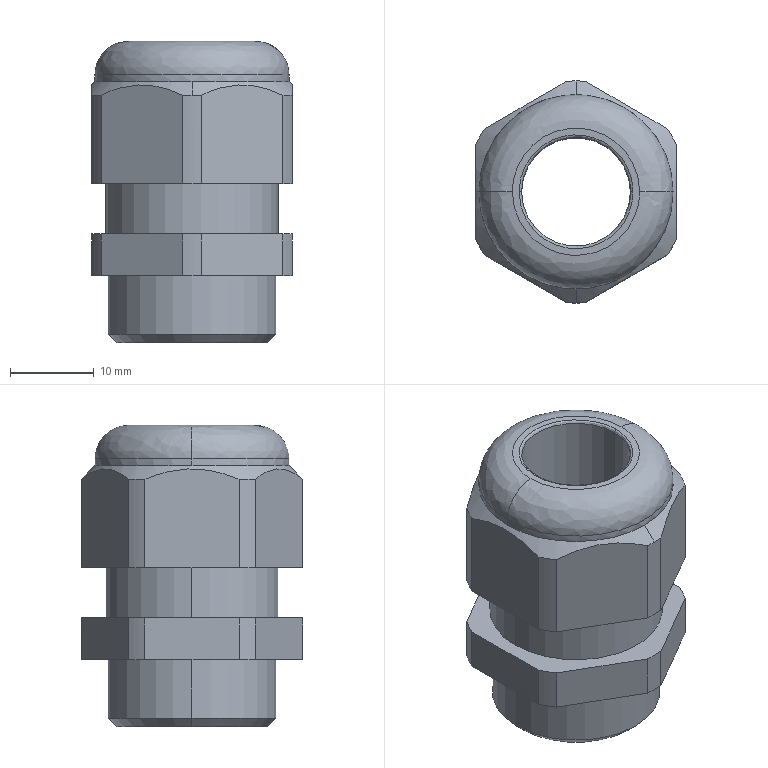Part | SolidWorks | features BaseBody 1 | 1 solid | 45 faces | box 24 x 26.5 x 36 mm | volume 9969 mm3 | cylinder 20 | plane 17 | spline 4 | cone 4 | commonest cylinder face diameters 26.5 x12 13 x2 20 x2 20.6 x2 23.2 x2